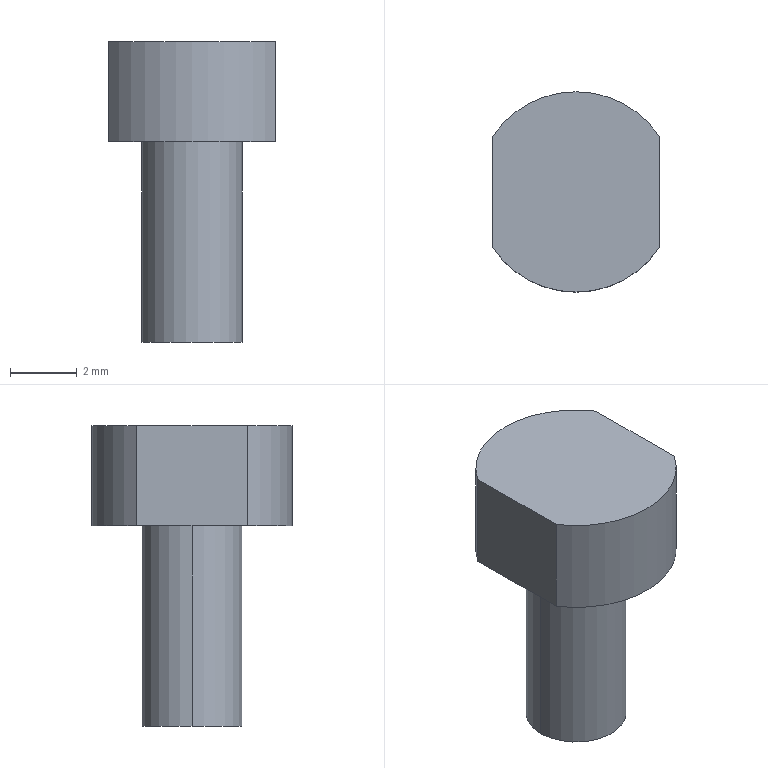Part | STEP file | M3 screw | 1 solid | 9 faces | box 5 x 6 x 9 mm | volume 120.482 mm3 | plane 5 | cylinder 4 | commonest cylinder face diameters 3 x2 6 x2
STEP:
#1=CARTESIAN_POINT('',(0.,0.,0.));
#2=DIRECTION('',(0.,0.,1.));
#3=DIRECTION('',(1.,0.,0.));
#4=AXIS2_PLACEMENT_3D('',#1,#2,#3);
#5=CARTESIAN_POINT('',(-1.5,0.,-6.));
#6=VERTEX_POINT('',#5);
#7=CARTESIAN_POINT('',(1.5,0.,-6.));
#8=VERTEX_POINT('',#7);
#9=CARTESIAN_POINT('',(0.,0.,-6.));
#10=DIRECTION('',(0.,0.,-1.));
#11=DIRECTION('',(-1.,0.,0.));
#12=AXIS2_PLACEMENT_3D('',#9,#10,#11);
#13=CIRCLE('',#12,1.5);
#14=CARTESIAN_POINT('',(0.,0.,-6.));
#15=DIRECTION('',(0.,0.,1.));
#16=DIRECTION('',(1.,0.,0.));
#17=AXIS2_PLACEMENT_3D('',#14,#15,#16);
#18=CYLINDRICAL_SURFACE('',#17,1.5);
#19=CARTESIAN_POINT('',(3.142,0.));
#20=DIRECTION('',(-1.,0.));
#21=VECTOR('',#20,1.);
#22=LINE('',#19,#21);
#23=(GEOMETRIC_REPRESENTATION_CONTEXT(2)PARAMETRIC_REPRESENTATION_CONTEXT()REPRESENTATION_CONTEXT('',''));
#24=DEFINITIONAL_REPRESENTATION('',(#22),#23);
#25=PCURVE('',#18,#24);
#26=CARTESIAN_POINT('',(0.,0.,-6.));
#27=DIRECTION('',(0.,0.,-1.));
#28=DIRECTION('',(-1.,0.,0.));
#29=AXIS2_PLACEMENT_3D('',#26,#27,#28);
#30=PLANE('',#29);
#31=CARTESIAN_POINT('',(0.,0.));
#32=DIRECTION('',(1.,0.));
#33=AXIS2_PLACEMENT_2D('',#31,#32);
#34=CIRCLE('',#33,1.5);
#35=(GEOMETRIC_REPRESENTATION_CONTEXT(2)PARAMETRIC_REPRESENTATION_CONTEXT()REPRESENTATION_CONTEXT('',''));
#36=DEFINITIONAL_REPRESENTATION('',(#34),#35);
#37=PCURVE('',#30,#36);
#38=SURFACE_CURVE('',#13,(#25,#37),.PCURVE_S1.);
#39=EDGE_CURVE('',#6,#8,#38,.T.);
#40=ORIENTED_EDGE('',*,*,#39,.F.);
#41=CARTESIAN_POINT('',(-1.5,0.,0.));
#42=VERTEX_POINT('',#41);
#43=CARTESIAN_POINT('',(-1.5,0.,-6.));
#44=DIRECTION('',(0.,0.,1.));
#45=VECTOR('',#44,1.);
#46=LINE('',#43,#45);
#47=CARTESIAN_POINT('',(3.142,0.));
#48=DIRECTION('',(0.,1.));
#49=VECTOR('',#48,1.);
#50=LINE('',#47,#49);
#51=(GEOMETRIC_REPRESENTATION_CONTEXT(2)PARAMETRIC_REPRESENTATION_CONTEXT()REPRESENTATION_CONTEXT('',''));
#52=DEFINITIONAL_REPRESENTATION('',(#50),#51);
#53=PCURVE('',#18,#52);
#54=CARTESIAN_POINT('',(0.,0.,-6.));
#55=DIRECTION('',(0.,0.,1.));
#56=DIRECTION('',(1.,0.,0.));
#57=AXIS2_PLACEMENT_3D('',#54,#55,#56);
#58=CYLINDRICAL_SURFACE('',#57,1.5);
#59=CARTESIAN_POINT('',(3.142,0.));
#60=DIRECTION('',(0.,1.));
#61=VECTOR('',#60,1.);
#62=LINE('',#59,#61);
#63=(GEOMETRIC_REPRESENTATION_CONTEXT(2)PARAMETRIC_REPRESENTATION_CONTEXT()REPRESENTATION_CONTEXT('',''));
#64=DEFINITIONAL_REPRESENTATION('',(#62),#63);
#65=PCURVE('',#58,#64);
#66=SURFACE_CURVE('',#46,(#53,#65),.PCURVE_S1.);
#67=EDGE_CURVE('',#6,#42,#66,.T.);
#68=ORIENTED_EDGE('',*,*,#67,.T.);
#69=CARTESIAN_POINT('',(1.5,0.,0.));
#70=VERTEX_POINT('',#69);
#71=CARTESIAN_POINT('',(0.,0.,0.));
#72=DIRECTION('',(0.,0.,-1.));
#73=DIRECTION('',(1.,0.,0.));
#74=AXIS2_PLACEMENT_3D('',#71,#72,#73);
#75=CIRCLE('',#74,1.5);
#76=CARTESIAN_POINT('',(6.283,6.));
#77=DIRECTION('',(-1.,0.));
#78=VECTOR('',#77,1.);
#79=LINE('',#76,#78);
#80=(GEOMETRIC_REPRESENTATION_CONTEXT(2)PARAMETRIC_REPRESENTATION_CONTEXT()REPRESENTATION_CONTEXT('',''));
#81=DEFINITIONAL_REPRESENTATION('',(#79),#80);
#82=PCURVE('',#18,#81);
#83=CARTESIAN_POINT('',(0.,0.,0.));
#84=DIRECTION('',(0.,0.,1.));
#85=DIRECTION('',(1.,0.,0.));
#86=AXIS2_PLACEMENT_3D('',#83,#84,#85);
#87=PLANE('',#86);
#88=CARTESIAN_POINT('',(1.5,0.));
#89=CARTESIAN_POINT('',(1.5,-2.598));
#90=CARTESIAN_POINT('',(-0.75,-1.299));
#91=CARTESIAN_POINT('',(-3.,0.));
#92=CARTESIAN_POINT('',(-0.75,1.299));
#93=CARTESIAN_POINT('',(1.5,2.598));
#94=CARTESIAN_POINT('',(1.5,0.));
#95=(BOUNDED_CURVE()B_SPLINE_CURVE(2,(#88,#89,#90,#91,#92,#93,#94),.UNSPECIFIED.,.T.,.F.)B_SPLINE_CURVE_WITH_KNOTS((1,2,2,2,2,1),(-2.094,0.,2.094,4.189,6.283,8.378),.UNSPECIFIED.)CURVE()GEOMETRIC_REPRESENTATION_ITEM()RATIONAL_B_SPLINE_CURVE((1.,0.5,1.,0.5,1.,0.5,1.))REPRESENTATION_ITEM(''));
#96=(GEOMETRIC_REPRESENTATION_CONTEXT(2)PARAMETRIC_REPRESENTATION_CONTEXT()REPRESENTATION_CONTEXT('',''));
#97=DEFINITIONAL_REPRESENTATION('',(#95),#96);
#98=PCURVE('',#87,#97);
#99=SURFACE_CURVE('',#75,(#82,#98),.PCURVE_S1.);
#100=EDGE_CURVE('',#42,#70,#99,.T.);
#101=ORIENTED_EDGE('',*,*,#100,.T.);
#102=CARTESIAN_POINT('',(1.5,0.,-6.));
#103=DIRECTION('',(0.,0.,1.));
#104=VECTOR('',#103,1.);
#105=LINE('',#102,#104);
#106=CARTESIAN_POINT('',(0.,0.));
#107=DIRECTION('',(0.,1.));
#108=VECTOR('',#107,1.);
#109=LINE('',#106,#108);
#110=(GEOMETRIC_REPRESENTATION_CONTEXT(2)PARAMETRIC_REPRESENTATION_CONTEXT()REPRESENTATION_CONTEXT('',''));
#111=DEFINITIONAL_REPRESENTATION('',(#109),#110);
#112=PCURVE('',#18,#111);
#113=CARTESIAN_POINT('',(6.283,0.));
#114=DIRECTION('',(0.,1.));
#115=VECTOR('',#114,1.);
#116=LINE('',#113,#115);
#117=(GEOMETRIC_REPRESENTATION_CONTEXT(2)PARAMETRIC_REPRESENTATION_CONTEXT()REPRESENTATION_CONTEXT('',''));
#118=DEFINITIONAL_REPRESENTATION('',(#116),#117);
#119=PCURVE('',#58,#118);
#120=SURFACE_CURVE('',#105,(#112,#119),.PCURVE_S1.);
#121=EDGE_CURVE('',#8,#70,#120,.T.);
#122=ORIENTED_EDGE('',*,*,#121,.F.);
#123=EDGE_LOOP('',(#40,#68,#101,#122));
#124=FACE_BOUND('',#123,.T.);
#125=ADVANCED_FACE('',(#124),#18,.T.);
#126=CARTESIAN_POINT('',(2.5,1.658,0.));
#127=VERTEX_POINT('',#126);
#128=CARTESIAN_POINT('',(-2.5,1.658,0.));
#129=VERTEX_POINT('',#128);
#130=CARTESIAN_POINT('',(0.,0.,0.));
#131=DIRECTION('',(0.,0.,1.));
#132=DIRECTION('',(1.,0.,0.));
#133=AXIS2_PLACEMENT_3D('',#130,#131,#132);
#134=CIRCLE('',#133,3.);
#135=CARTESIAN_POINT('',(0.,0.,3.));
#136=DIRECTION('',(0.,0.,-1.));
#137=DIRECTION('',(-1.,0.,0.));
#138=AXIS2_PLACEMENT_3D('',#135,#136,#137);
#139=CYLINDRICAL_SURFACE('',#138,3.);
#140=CARTESIAN_POINT('',(3.142,3.));
#141=DIRECTION('',(-1.,0.));
#142=VECTOR('',#141,1.);
#143=LINE('',#140,#142);
#144=(GEOMETRIC_REPRESENTATION_CONTEXT(2)PARAMETRIC_REPRESENTATION_CONTEXT()REPRESENTATION_CONTEXT('',''));
#145=DEFINITIONAL_REPRESENTATION('',(#143),#144);
#146=PCURVE('',#139,#145);
#147=CARTESIAN_POINT('',(0.,0.));
#148=DIRECTION('',(1.,0.));
#149=AXIS2_PLACEMENT_2D('',#147,#148);
#150=CIRCLE('',#149,3.);
#151=(GEOMETRIC_REPRESENTATION_CONTEXT(2)PARAMETRIC_REPRESENTATION_CONTEXT()REPRESENTATION_CONTEXT('',''));
#152=DEFINITIONAL_REPRESENTATION('',(#150),#151);
#153=PCURVE('',#87,#152);
#154=SURFACE_CURVE('',#134,(#146,#153),.PCURVE_S1.);
#155=EDGE_CURVE('',#127,#129,#154,.T.);
#156=ORIENTED_EDGE('',*,*,#155,.T.);
#157=CARTESIAN_POINT('',(-2.5,1.658,3.));
#158=VERTEX_POINT('',#157);
#159=CARTESIAN_POINT('',(-2.5,1.658,-6.));
#160=DIRECTION('',(0.,0.,1.));
#161=VECTOR('',#160,1.);
#162=LINE('',#159,#161);
#163=CARTESIAN_POINT('',(0.5857,9.));
#164=DIRECTION('',(0.,-1.));
#165=VECTOR('',#164,1.);
#166=LINE('',#163,#165);
#167=(GEOMETRIC_REPRESENTATION_CONTEXT(2)PARAMETRIC_REPRESENTATION_CONTEXT()REPRESENTATION_CONTEXT('',''));
#168=DEFINITIONAL_REPRESENTATION('',(#166),#167);
#169=PCURVE('',#139,#168);
#170=CARTESIAN_POINT('',(-2.5,1.658,-6.));
#171=DIRECTION('',(1.,0.,0.));
#172=DIRECTION('',(0.,0.,-1.));
#173=AXIS2_PLACEMENT_3D('',#170,#171,#172);
#174=PLANE('',#173);
#175=CARTESIAN_POINT('',(0.,0.));
#176=DIRECTION('',(-1.,0.));
#177=VECTOR('',#176,1.);
#178=LINE('',#175,#177);
#179=(GEOMETRIC_REPRESENTATION_CONTEXT(2)PARAMETRIC_REPRESENTATION_CONTEXT()REPRESENTATION_CONTEXT('',''));
#180=DEFINITIONAL_REPRESENTATION('',(#178),#179);
#181=PCURVE('',#174,#180);
#182=SURFACE_CURVE('',#162,(#169,#181),.PCURVE_S1.);
#183=EDGE_CURVE('',#129,#158,#182,.T.);
#184=ORIENTED_EDGE('',*,*,#183,.T.);
#185=CARTESIAN_POINT('',(2.5,1.658,3.));
#186=VERTEX_POINT('',#185);
#187=CARTESIAN_POINT('',(0.,0.,3.));
#188=DIRECTION('',(0.,0.,1.));
#189=DIRECTION('',(1.,0.,0.));
#190=AXIS2_PLACEMENT_3D('',#187,#188,#189);
#191=CIRCLE('',#190,3.);
#192=CARTESIAN_POINT('',(3.142,0.));
#193=DIRECTION('',(-1.,0.));
#194=VECTOR('',#193,1.);
#195=LINE('',#192,#194);
#196=(GEOMETRIC_REPRESENTATION_CONTEXT(2)PARAMETRIC_REPRESENTATION_CONTEXT()REPRESENTATION_CONTEXT('',''));
#197=DEFINITIONAL_REPRESENTATION('',(#195),#196);
#198=PCURVE('',#139,#197);
#199=CARTESIAN_POINT('',(0.,0.,3.));
#200=DIRECTION('',(0.,0.,1.));
#201=DIRECTION('',(1.,0.,0.));
#202=AXIS2_PLACEMENT_3D('',#199,#200,#201);
#203=PLANE('',#202);
#204=CARTESIAN_POINT('',(0.,0.));
#205=DIRECTION('',(1.,0.));
#206=AXIS2_PLACEMENT_2D('',#204,#205);
#207=CIRCLE('',#206,3.);
#208=(GEOMETRIC_REPRESENTATION_CONTEXT(2)PARAMETRIC_REPRESENTATION_CONTEXT()REPRESENTATION_CONTEXT('',''));
#209=DEFINITIONAL_REPRESENTATION('',(#207),#208);
#210=PCURVE('',#203,#209);
#211=SURFACE_CURVE('',#191,(#198,#210),.PCURVE_S1.);
#212=EDGE_CURVE('',#186,#158,#211,.T.);
#213=ORIENTED_EDGE('',*,*,#212,.F.);
#214=CARTESIAN_POINT('',(2.5,1.658,-6.));
#215=DIRECTION('',(0.,0.,1.));
#216=VECTOR('',#215,1.);
#217=LINE('',#214,#216);
#218=CARTESIAN_POINT('',(2.556,9.));
#219=DIRECTION('',(0.,-1.));
#220=VECTOR('',#219,1.);
#221=LINE('',#218,#220);
#222=(GEOMETRIC_REPRESENTATION_CONTEXT(2)PARAMETRIC_REPRESENTATION_CONTEXT()REPRESENTATION_CONTEXT('',''));
#223=DEFINITIONAL_REPRESENTATION('',(#221),#222);
#224=PCURVE('',#139,#223);
#225=CARTESIAN_POINT('',(2.5,1.658,-6.));
#226=DIRECTION('',(-1.,0.,0.));
#227=DIRECTION('',(0.,0.,1.));
#228=AXIS2_PLACEMENT_3D('',#225,#226,#227);
#229=PLANE('',#228);
#230=CARTESIAN_POINT('',(0.,0.));
#231=DIRECTION('',(1.,0.));
#232=VECTOR('',#231,1.);
#233=LINE('',#230,#232);
#234=(GEOMETRIC_REPRESENTATION_CONTEXT(2)PARAMETRIC_REPRESENTATION_CONTEXT()REPRESENTATION_CONTEXT('',''));
#235=DEFINITIONAL_REPRESENTATION('',(#233),#234);
#236=PCURVE('',#229,#235);
#237=SURFACE_CURVE('',#217,(#224,#236),.PCURVE_S1.);
#238=EDGE_CURVE('',#127,#186,#237,.T.);
#239=ORIENTED_EDGE('',*,*,#238,.F.);
#240=EDGE_LOOP('',(#156,#184,#213,#239));
#241=FACE_BOUND('',#240,.T.);
#242=ADVANCED_FACE('',(#241),#139,.T.);
#243=CARTESIAN_POINT('',(-2.5,-1.658,0.));
#244=VERTEX_POINT('',#243);
#245=CARTESIAN_POINT('',(2.5,-1.658,0.));
#246=VERTEX_POINT('',#245);
#247=CARTESIAN_POINT('',(0.,0.,0.));
#248=DIRECTION('',(0.,0.,1.));
#249=DIRECTION('',(1.,0.,0.));
#250=AXIS2_PLACEMENT_3D('',#247,#248,#249);
#251=CIRCLE('',#250,3.);
#252=CARTESIAN_POINT('',(0.,0.));
#253=DIRECTION('',(1.,0.));
#254=AXIS2_PLACEMENT_2D('',#252,#253);
#255=CIRCLE('',#254,3.);
#256=(GEOMETRIC_REPRESENTATION_CONTEXT(2)PARAMETRIC_REPRESENTATION_CONTEXT()REPRESENTATION_CONTEXT('',''));
#257=DEFINITIONAL_REPRESENTATION('',(#255),#256);
#258=PCURVE('',#87,#257);
#259=CARTESIAN_POINT('',(0.,0.,3.));
#260=DIRECTION('',(0.,0.,-1.));
#261=DIRECTION('',(-1.,0.,0.));
#262=AXIS2_PLACEMENT_3D('',#259,#260,#261);
#263=CYLINDRICAL_SURFACE('',#262,3.);
#264=CARTESIAN_POINT('',(9.425,3.));
#265=DIRECTION('',(-1.,0.));
#266=VECTOR('',#265,1.);
#267=LINE('',#264,#266);
#268=(GEOMETRIC_REPRESENTATION_CONTEXT(2)PARAMETRIC_REPRESENTATION_CONTEXT()REPRESENTATION_CONTEXT('',''));
#269=DEFINITIONAL_REPRESENTATION('',(#267),#268);
#270=PCURVE('',#263,#269);
#271=SURFACE_CURVE('',#251,(#258,#270),.PCURVE_S1.);
#272=EDGE_CURVE('',#244,#246,#271,.T.);
#273=ORIENTED_EDGE('',*,*,#272,.F.);
#274=CARTESIAN_POINT('',(-2.5,0.,0.));
#275=DIRECTION('',(0.,1.,0.));
#276=VECTOR('',#275,1.);
#277=LINE('',#274,#276);
#278=CARTESIAN_POINT('',(-2.5,0.));
#279=DIRECTION('',(0.,1.));
#280=VECTOR('',#279,1.);
#281=LINE('',#278,#280);
#282=(GEOMETRIC_REPRESENTATION_CONTEXT(2)PARAMETRIC_REPRESENTATION_CONTEXT()REPRESENTATION_CONTEXT('',''));
#283=DEFINITIONAL_REPRESENTATION('',(#281),#282);
#284=PCURVE('',#87,#283);
#285=CARTESIAN_POINT('',(-6.,-1.658));
#286=DIRECTION('',(0.,1.));
#287=VECTOR('',#286,1.);
#288=LINE('',#285,#287);
#289=(GEOMETRIC_REPRESENTATION_CONTEXT(2)PARAMETRIC_REPRESENTATION_CONTEXT()REPRESENTATION_CONTEXT('',''));
#290=DEFINITIONAL_REPRESENTATION('',(#288),#289);
#291=PCURVE('',#174,#290);
#292=SURFACE_CURVE('',#277,(#284,#291),.PCURVE_S1.);
#293=EDGE_CURVE('',#244,#129,#292,.T.);
#294=ORIENTED_EDGE('',*,*,#293,.T.);
#295=ORIENTED_EDGE('',*,*,#155,.F.);
#296=CARTESIAN_POINT('',(2.5,0.,0.));
#297=DIRECTION('',(0.,-1.,0.));
#298=VECTOR('',#297,1.);
#299=LINE('',#296,#298);
#300=CARTESIAN_POINT('',(2.5,0.));
#301=DIRECTION('',(0.,-1.));
#302=VECTOR('',#301,1.);
#303=LINE('',#300,#302);
#304=(GEOMETRIC_REPRESENTATION_CONTEXT(2)PARAMETRIC_REPRESENTATION_CONTEXT()REPRESENTATION_CONTEXT('',''));
#305=DEFINITIONAL_REPRESENTATION('',(#303),#304);
#306=PCURVE('',#87,#305);
#307=CARTESIAN_POINT('',(6.,-1.658));
#308=DIRECTION('',(0.,-1.));
#309=VECTOR('',#308,1.);
#310=LINE('',#307,#309);
#311=(GEOMETRIC_REPRESENTATION_CONTEXT(2)PARAMETRIC_REPRESENTATION_CONTEXT()REPRESENTATION_CONTEXT('',''));
#312=DEFINITIONAL_REPRESENTATION('',(#310),#311);
#313=PCURVE('',#229,#312);
#314=SURFACE_CURVE('',#299,(#306,#313),.PCURVE_S1.);
#315=EDGE_CURVE('',#127,#246,#314,.T.);
#316=ORIENTED_EDGE('',*,*,#315,.T.);
#317=EDGE_LOOP('',(#273,#294,#295,#316));
#318=FACE_BOUND('',#317,.T.);
#319=CARTESIAN_POINT('',(0.,0.,0.));
#320=DIRECTION('',(0.,0.,-1.));
#321=DIRECTION('',(1.,0.,0.));
#322=AXIS2_PLACEMENT_3D('',#319,#320,#321);
#323=CIRCLE('',#322,1.5);
#324=CARTESIAN_POINT('',(1.5,0.));
#325=CARTESIAN_POINT('',(1.5,-2.598));
#326=CARTESIAN_POINT('',(-0.75,-1.299));
#327=CARTESIAN_POINT('',(-3.,0.));
#328=CARTESIAN_POINT('',(-0.75,1.299));
#329=CARTESIAN_POINT('',(1.5,2.598));
#330=CARTESIAN_POINT('',(1.5,0.));
#331=(BOUNDED_CURVE()B_SPLINE_CURVE(2,(#324,#325,#326,#327,#328,#329,#330),.UNSPECIFIED.,.T.,.F.)B_SPLINE_CURVE_WITH_KNOTS((1,2,2,2,2,1),(-2.094,0.,2.094,4.189,6.283,8.378),.UNSPECIFIED.)CURVE()GEOMETRIC_REPRESENTATION_ITEM()RATIONAL_B_SPLINE_CURVE((1.,0.5,1.,0.5,1.,0.5,1.))REPRESENTATION_ITEM(''));
#332=(GEOMETRIC_REPRESENTATION_CONTEXT(2)PARAMETRIC_REPRESENTATION_CONTEXT()REPRESENTATION_CONTEXT('',''));
#333=DEFINITIONAL_REPRESENTATION('',(#331),#332);
#334=PCURVE('',#87,#333);
#335=CARTESIAN_POINT('',(6.283,6.));
#336=DIRECTION('',(-1.,0.));
#337=VECTOR('',#336,1.);
#338=LINE('',#335,#337);
#339=(GEOMETRIC_REPRESENTATION_CONTEXT(2)PARAMETRIC_REPRESENTATION_CONTEXT()REPRESENTATION_CONTEXT('',''));
#340=DEFINITIONAL_REPRESENTATION('',(#338),#339);
#341=PCURVE('',#58,#340);
#342=SURFACE_CURVE('',#323,(#334,#341),.PCURVE_S1.);
#343=EDGE_CURVE('',#70,#42,#342,.T.);
#344=ORIENTED_EDGE('',*,*,#343,.F.);
#345=ORIENTED_EDGE('',*,*,#100,.F.);
#346=EDGE_LOOP('',(#344,#345));
#347=FACE_BOUND('',#346,.T.);
#348=ADVANCED_FACE('',(#318,#347),#87,.F.);
#349=CARTESIAN_POINT('',(-2.5,-1.658,3.));
#350=VERTEX_POINT('',#349);
#351=CARTESIAN_POINT('',(2.5,-1.658,3.));
#352=VERTEX_POINT('',#351);
#353=CARTESIAN_POINT('',(0.,0.,3.));
#354=DIRECTION('',(0.,0.,1.));
#355=DIRECTION('',(1.,0.,0.));
#356=AXIS2_PLACEMENT_3D('',#353,#354,#355);
#357=CIRCLE('',#356,3.);
#358=CARTESIAN_POINT('',(9.425,0.));
#359=DIRECTION('',(-1.,0.));
#360=VECTOR('',#359,1.);
#361=LINE('',#358,#360);
#362=(GEOMETRIC_REPRESENTATION_CONTEXT(2)PARAMETRIC_REPRESENTATION_CONTEXT()REPRESENTATION_CONTEXT('',''));
#363=DEFINITIONAL_REPRESENTATION('',(#361),#362);
#364=PCURVE('',#263,#363);
#365=CARTESIAN_POINT('',(0.,0.));
#366=DIRECTION('',(1.,0.));
#367=AXIS2_PLACEMENT_2D('',#365,#366);
#368=CIRCLE('',#367,3.);
#369=(GEOMETRIC_REPRESENTATION_CONTEXT(2)PARAMETRIC_REPRESENTATION_CONTEXT()REPRESENTATION_CONTEXT('',''));
#370=DEFINITIONAL_REPRESENTATION('',(#368),#369);
#371=PCURVE('',#203,#370);
#372=SURFACE_CURVE('',#357,(#364,#371),.PCURVE_S1.);
#373=EDGE_CURVE('',#350,#352,#372,.T.);
#374=ORIENTED_EDGE('',*,*,#373,.F.);
#375=CARTESIAN_POINT('',(-2.5,-1.658,-6.));
#376=DIRECTION('',(0.,0.,1.));
#377=VECTOR('',#376,1.);
#378=LINE('',#375,#377);
#379=CARTESIAN_POINT('',(5.697,9.));
#380=DIRECTION('',(0.,-1.));
#381=VECTOR('',#380,1.);
#382=LINE('',#379,#381);
#383=(GEOMETRIC_REPRESENTATION_CONTEXT(2)PARAMETRIC_REPRESENTATION_CONTEXT()REPRESENTATION_CONTEXT('',''));
#384=DEFINITIONAL_REPRESENTATION('',(#382),#383);
#385=PCURVE('',#263,#384);
#386=CARTESIAN_POINT('',(0.,-3.317));
#387=DIRECTION('',(-1.,0.));
#388=VECTOR('',#387,1.);
#389=LINE('',#386,#388);
#390=(GEOMETRIC_REPRESENTATION_CONTEXT(2)PARAMETRIC_REPRESENTATION_CONTEXT()REPRESENTATION_CONTEXT('',''));
#391=DEFINITIONAL_REPRESENTATION('',(#389),#390);
#392=PCURVE('',#174,#391);
#393=SURFACE_CURVE('',#378,(#385,#392),.PCURVE_S1.);
#394=EDGE_CURVE('',#244,#350,#393,.T.);
#395=ORIENTED_EDGE('',*,*,#394,.F.);
#396=ORIENTED_EDGE('',*,*,#272,.T.);
#397=CARTESIAN_POINT('',(2.5,-1.658,-6.));
#398=DIRECTION('',(0.,0.,1.));
#399=VECTOR('',#398,1.);
#400=LINE('',#397,#399);
#401=CARTESIAN_POINT('',(3.727,9.));
#402=DIRECTION('',(0.,-1.));
#403=VECTOR('',#402,1.);
#404=LINE('',#401,#403);
#405=(GEOMETRIC_REPRESENTATION_CONTEXT(2)PARAMETRIC_REPRESENTATION_CONTEXT()REPRESENTATION_CONTEXT('',''));
#406=DEFINITIONAL_REPRESENTATION('',(#404),#405);
#407=PCURVE('',#263,#406);
#408=CARTESIAN_POINT('',(0.,-3.317));
#409=DIRECTION('',(1.,0.));
#410=VECTOR('',#409,1.);
#411=LINE('',#408,#410);
#412=(GEOMETRIC_REPRESENTATION_CONTEXT(2)PARAMETRIC_REPRESENTATION_CONTEXT()REPRESENTATION_CONTEXT('',''));
#413=DEFINITIONAL_REPRESENTATION('',(#411),#412);
#414=PCURVE('',#229,#413);
#415=SURFACE_CURVE('',#400,(#407,#414),.PCURVE_S1.);
#416=EDGE_CURVE('',#246,#352,#415,.T.);
#417=ORIENTED_EDGE('',*,*,#416,.T.);
#418=EDGE_LOOP('',(#374,#395,#396,#417));
#419=FACE_BOUND('',#418,.T.);
#420=ADVANCED_FACE('',(#419),#263,.T.);
#421=CARTESIAN_POINT('',(-2.5,1.658,3.));
#422=DIRECTION('',(0.,1.,0.));
#423=VECTOR('',#422,1.);
#424=LINE('',#421,#423);
#425=CARTESIAN_POINT('',(-2.5,1.658));
#426=DIRECTION('',(0.,1.));
#427=VECTOR('',#426,1.);
#428=LINE('',#425,#427);
#429=(GEOMETRIC_REPRESENTATION_CONTEXT(2)PARAMETRIC_REPRESENTATION_CONTEXT()REPRESENTATION_CONTEXT('',''));
#430=DEFINITIONAL_REPRESENTATION('',(#428),#429);
#431=PCURVE('',#203,#430);
#432=CARTESIAN_POINT('',(-9.,0.));
#433=DIRECTION('',(0.,1.));
#434=VECTOR('',#433,1.);
#435=LINE('',#432,#434);
#436=(GEOMETRIC_REPRESENTATION_CONTEXT(2)PARAMETRIC_REPRESENTATION_CONTEXT()REPRESENTATION_CONTEXT('',''));
#437=DEFINITIONAL_REPRESENTATION('',(#435),#436);
#438=PCURVE('',#174,#437);
#439=SURFACE_CURVE('',#424,(#431,#438),.PCURVE_S1.);
#440=EDGE_CURVE('',#350,#158,#439,.T.);
#441=ORIENTED_EDGE('',*,*,#440,.F.);
#442=ORIENTED_EDGE('',*,*,#373,.T.);
#443=CARTESIAN_POINT('',(2.5,1.658,3.));
#444=DIRECTION('',(0.,-1.,0.));
#445=VECTOR('',#444,1.);
#446=LINE('',#443,#445);
#447=CARTESIAN_POINT('',(2.5,1.658));
#448=DIRECTION('',(0.,-1.));
#449=VECTOR('',#448,1.);
#450=LINE('',#447,#449);
#451=(GEOMETRIC_REPRESENTATION_CONTEXT(2)PARAMETRIC_REPRESENTATION_CONTEXT()REPRESENTATION_CONTEXT('',''));
#452=DEFINITIONAL_REPRESENTATION('',(#450),#451);
#453=PCURVE('',#203,#452);
#454=CARTESIAN_POINT('',(9.,0.));
#455=DIRECTION('',(0.,-1.));
#456=VECTOR('',#455,1.);
#457=LINE('',#454,#456);
#458=(GEOMETRIC_REPRESENTATION_CONTEXT(2)PARAMETRIC_REPRESENTATION_CONTEXT()REPRESENTATION_CONTEXT('',''));
#459=DEFINITIONAL_REPRESENTATION('',(#457),#458);
#460=PCURVE('',#229,#459);
#461=SURFACE_CURVE('',#446,(#453,#460),.PCURVE_S1.);
#462=EDGE_CURVE('',#186,#352,#461,.T.);
#463=ORIENTED_EDGE('',*,*,#462,.F.);
#464=ORIENTED_EDGE('',*,*,#212,.T.);
#465=EDGE_LOOP('',(#441,#442,#463,#464));
#466=FACE_BOUND('',#465,.T.);
#467=ADVANCED_FACE('',(#466),#203,.T.);
#468=ORIENTED_EDGE('',*,*,#67,.F.);
#469=CARTESIAN_POINT('',(0.,0.,-6.));
#470=DIRECTION('',(0.,0.,-1.));
#471=DIRECTION('',(-1.,0.,0.));
#472=AXIS2_PLACEMENT_3D('',#469,#470,#471);
#473=CIRCLE('',#472,1.5);
#474=CARTESIAN_POINT('',(9.425,0.));
#475=DIRECTION('',(-1.,0.));
#476=VECTOR('',#475,1.);
#477=LINE('',#474,#476);
#478=(GEOMETRIC_REPRESENTATION_CONTEXT(2)PARAMETRIC_REPRESENTATION_CONTEXT()REPRESENTATION_CONTEXT('',''));
#479=DEFINITIONAL_REPRESENTATION('',(#477),#478);
#480=PCURVE('',#58,#479);
#481=CARTESIAN_POINT('',(0.,0.));
#482=DIRECTION('',(1.,0.));
#483=AXIS2_PLACEMENT_2D('',#481,#482);
#484=CIRCLE('',#483,1.5);
#485=(GEOMETRIC_REPRESENTATION_CONTEXT(2)PARAMETRIC_REPRESENTATION_CONTEXT()REPRESENTATION_CONTEXT('',''));
#486=DEFINITIONAL_REPRESENTATION('',(#484),#485);
#487=PCURVE('',#30,#486);
#488=SURFACE_CURVE('',#473,(#480,#487),.PCURVE_S1.);
#489=EDGE_CURVE('',#8,#6,#488,.T.);
#490=ORIENTED_EDGE('',*,*,#489,.F.);
#491=ORIENTED_EDGE('',*,*,#121,.T.);
#492=ORIENTED_EDGE('',*,*,#343,.T.);
#493=EDGE_LOOP('',(#468,#490,#491,#492));
#494=FACE_BOUND('',#493,.T.);
#495=ADVANCED_FACE('',(#494),#58,.T.);
#496=ORIENTED_EDGE('',*,*,#489,.T.);
#497=ORIENTED_EDGE('',*,*,#39,.T.);
#498=EDGE_LOOP('',(#496,#497));
#499=FACE_BOUND('',#498,.T.);
#500=ADVANCED_FACE('',(#499),#30,.T.);
#501=ORIENTED_EDGE('',*,*,#238,.T.);
#502=ORIENTED_EDGE('',*,*,#462,.T.);
#503=ORIENTED_EDGE('',*,*,#416,.F.);
#504=ORIENTED_EDGE('',*,*,#315,.F.);
#505=EDGE_LOOP('',(#501,#502,#503,#504));
#506=FACE_BOUND('',#505,.T.);
#507=ADVANCED_FACE('',(#506),#229,.F.);
#508=ORIENTED_EDGE('',*,*,#394,.T.);
#509=ORIENTED_EDGE('',*,*,#440,.T.);
#510=ORIENTED_EDGE('',*,*,#183,.F.);
#511=ORIENTED_EDGE('',*,*,#293,.F.);
#512=EDGE_LOOP('',(#508,#509,#510,#511));
#513=FACE_BOUND('',#512,.T.);
#514=ADVANCED_FACE('',(#513),#174,.F.);
#515=CLOSED_SHELL('',(#125,#242,#348,#420,#467,#495,#500,#507,#514));
#516=MANIFOLD_SOLID_BREP('',#515);
#517=(LENGTH_UNIT()NAMED_UNIT(*)SI_UNIT(.MILLI.,.METRE.));
#518=UNCERTAINTY_MEASURE_WITH_UNIT(LENGTH_MEASURE(0.0000001),#517,'','');
#519=(NAMED_UNIT(*)PLANE_ANGLE_UNIT()SI_UNIT($,.RADIAN.));
#520=(NAMED_UNIT(*)SI_UNIT($,.STERADIAN.)SOLID_ANGLE_UNIT());
#521=(GEOMETRIC_REPRESENTATION_CONTEXT(3)GLOBAL_UNCERTAINTY_ASSIGNED_CONTEXT((#518))GLOBAL_UNIT_ASSIGNED_CONTEXT((#517,#519,#520))REPRESENTATION_CONTEXT('',''));
#522=ADVANCED_BREP_SHAPE_REPRESENTATION('',(#4,#516),#521);